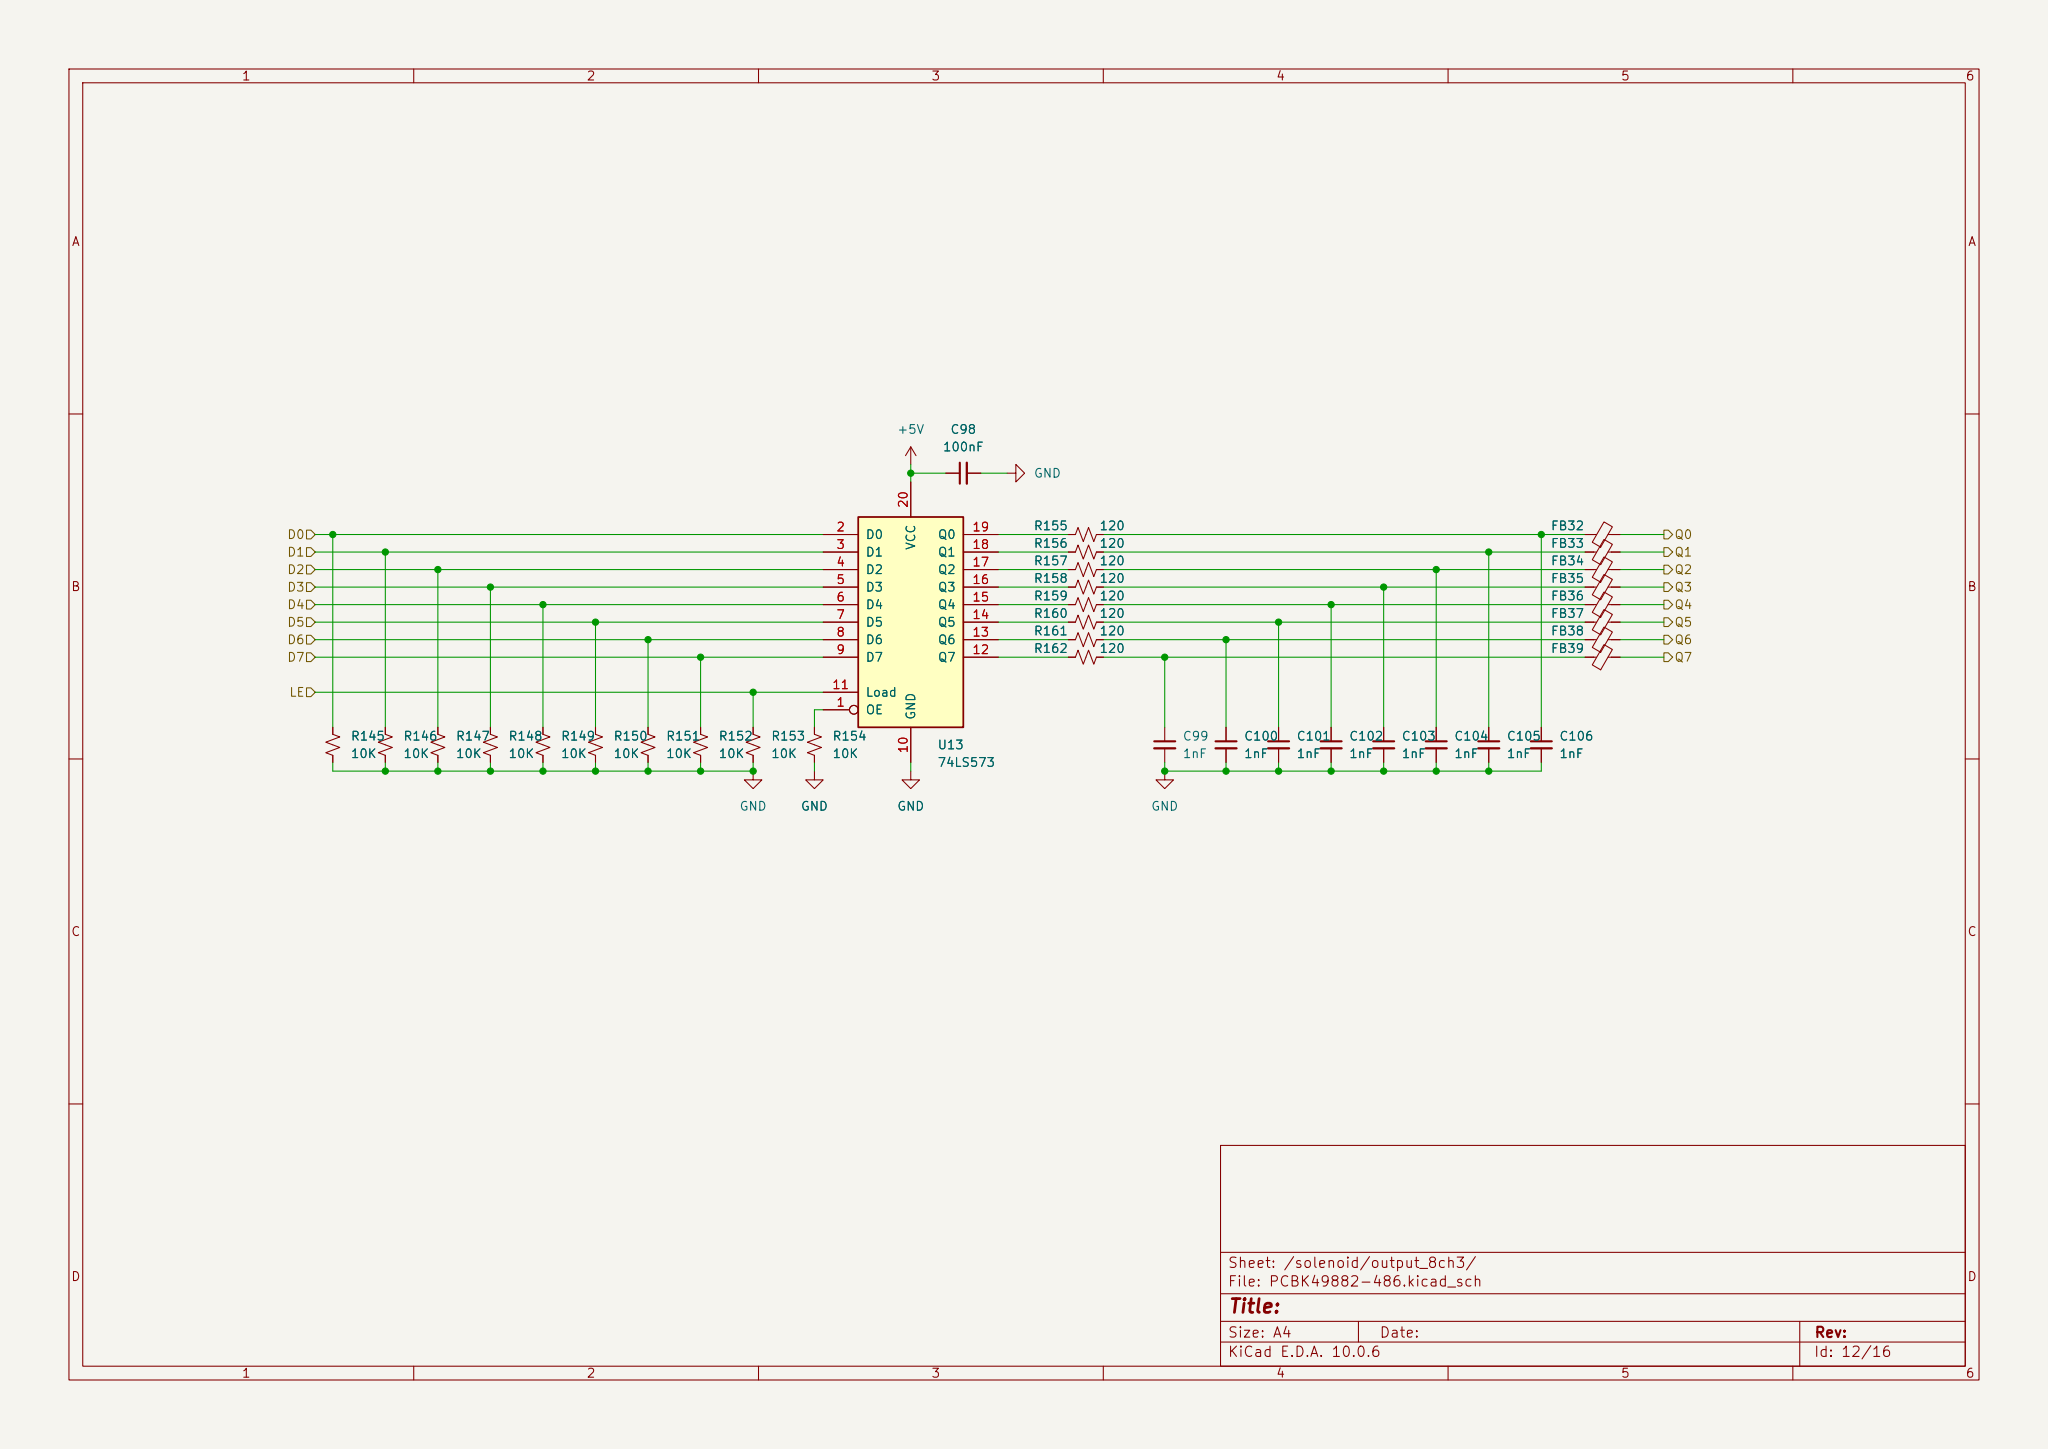Circuit board | KiCad | 536 parts | 438 nets | one sheet of the schematic
Parts on this sheet (reference | value | footprint):
C100
C101
C102
C103
C104
C105
C106
C98 | 100nF | Capacitor_SMD:C_0603_1608Metric
C99
FB32
FB33
FB34
FB35
FB36
FB37
FB38
FB39
R145
R146
R147
R148
R149
R150
R151
R152
R153
R154
R155
R156
R157
R158
R159
R160
R161
R162
U13
Nets of these parts (net: part-pin ...):
+5V: C98-1 U13-20
/core_board_b2b/PA0_C{slash}ADC12_INP0: R145-1 U13-2
/core_board_b2b/PA0{slash}WAKE_UP{slash}ADC1_INP16: R153-1 U13-11
/core_board_b2b/PA1_C{slash}ADC12_INP1: R146-1 U13-3
/core_board_b2b/PA3{slash}ADC12_INP15: R149-1 U13-6
/core_board_b2b/PA4{slash}ADC12_INP18: R150-1 U13-7
/core_board_b2b/PA5{slash}ADC12_INP19: R151-1 U13-8
/core_board_b2b/PA6{slash}ADC12_INP3: R152-1 U13-9
/core_board_b2b/PC2_C{slash}ADC3_INP0: R147-1 U13-4
/core_board_b2b/PC3_C{slash}ADC3_INP1: R148-1 U13-5
/solenoid/OUTPUT24: FB32-2
/solenoid/OUTPUT25: FB33-2
/solenoid/OUTPUT26: FB34-2
/solenoid/OUTPUT27: FB35-2
/solenoid/OUTPUT28: FB36-2
/solenoid/OUTPUT29: FB37-2
/solenoid/OUTPUT30: FB38-2
/solenoid/OUTPUT31: FB39-2
GND: C98-2 C99-2 C100-2 C101-2 C102-2 C103-2 C104-2 C105-2 C106-2 R145-2 R146-2 R147-2 R148-2 R149-2 R150-2 R151-2 R152-2 R153-2 R154-2 U13-10
Net-(C99-Pad1): C99-1 FB39-1 R162-2
Net-(C100-Pad1): C100-1 FB38-1 R161-2
Net-(C101-Pad1): C101-1 FB37-1 R160-2
Net-(C102-Pad1): C102-1 FB36-1 R159-2
Net-(C103-Pad1): C103-1 FB35-1 R158-2
Net-(C104-Pad1): C104-1 FB34-1 R157-2
Net-(C105-Pad1): C105-1 FB33-1 R156-2
Net-(C106-Pad1): C106-1 FB32-1 R155-2
Net-(U13-OE): R154-1 U13-1
Net-(U13-Q0): R155-1 U13-19
Net-(U13-Q1): R156-1 U13-18
Net-(U13-Q2): R157-1 U13-17
Net-(U13-Q3): R158-1 U13-16
Net-(U13-Q4): R159-1 U13-15
Net-(U13-Q5): R160-1 U13-14
Net-(U13-Q6): R161-1 U13-13
Net-(U13-Q7): R162-1 U13-12